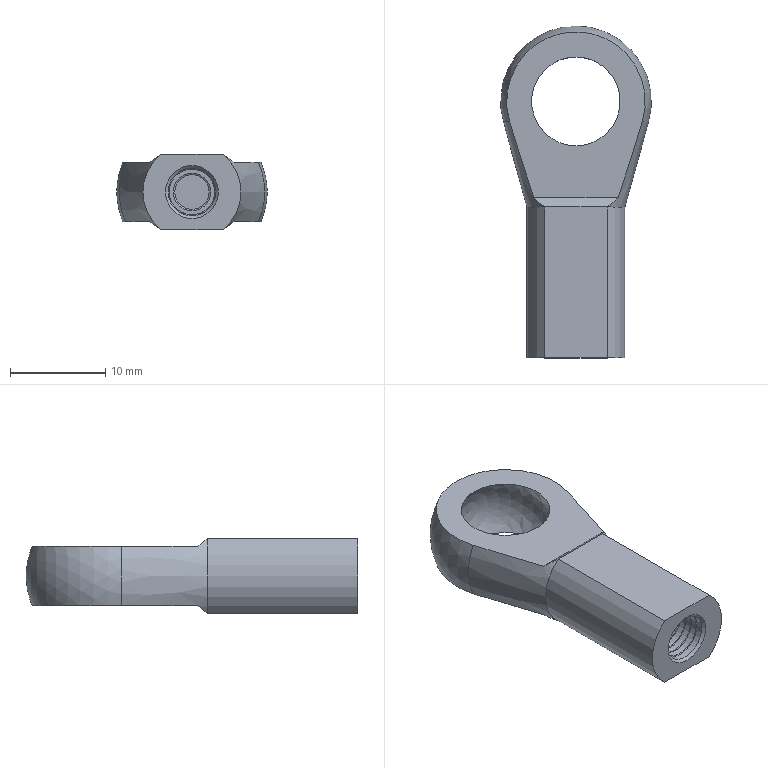Part | NX | features MG0312 tapped 1064K711(1064K711) 2 | 1 solid | 63 faces | box 15.875 x 34.925 x 7.925 mm | volume 1838 mm3 | cone 34 | cylinder 18 | plane 9 | sphere 2 | commonest cylinder face diameters 4.826 x15 10.312 x2 5 x1
STEP:
#1=CARTESIAN_POINT('',(6.982,12.167,-3.124));
#2=VERTEX_POINT('',#1);
#3=CARTESIAN_POINT('',(4.445,4.174,-3.124));
#4=VERTEX_POINT('',#3);
#5=CARTESIAN_POINT('',(6.982,12.167,-3.124));
#6=CARTESIAN_POINT('',(6.17,9.492,-3.124));
#7=CARTESIAN_POINT('',(5.342,6.821,-3.124));
#8=CARTESIAN_POINT('',(4.445,4.174,-3.124));
#9=B_SPLINE_CURVE_WITH_KNOTS('',3,(#5,#6,#7,#8),.UNSPECIFIED.,.F.,.F.,(4,4),(0.0111,0.01949),.UNSPECIFIED.);
#10=EDGE_CURVE('',#2,#4,#9,.T.);
#11=ORIENTED_EDGE('',*,*,#10,.F.);
#12=CARTESIAN_POINT('',(6.982,12.167,3.124));
#13=VERTEX_POINT('',#12);
#14=CARTESIAN_POINT('',(0.,12.167,0.));
#15=DIRECTION('',(0.,-1.,0.));
#16=DIRECTION('',(0.,0.,-1.));
#17=AXIS2_PLACEMENT_3D('',#14,#15,#16);
#18=CIRCLE('',#17,7.649);
#19=EDGE_CURVE('',#2,#13,#18,.T.);
#20=ORIENTED_EDGE('',*,*,#19,.T.);
#21=CARTESIAN_POINT('',(4.445,4.174,3.124));
#22=VERTEX_POINT('',#21);
#23=CARTESIAN_POINT('',(4.445,4.174,3.124));
#24=CARTESIAN_POINT('',(5.342,6.822,3.124));
#25=CARTESIAN_POINT('',(6.17,9.492,3.124));
#26=CARTESIAN_POINT('',(6.982,12.167,3.124));
#27=B_SPLINE_CURVE_WITH_KNOTS('',3,(#23,#24,#25,#26),.UNSPECIFIED.,.F.,.F.,(4,4),(0.03896,0.04741),.UNSPECIFIED.);
#28=EDGE_CURVE('',#22,#13,#27,.T.);
#29=ORIENTED_EDGE('',*,*,#28,.F.);
#30=CARTESIAN_POINT('',(3.299,3.175,3.962));
#31=VERTEX_POINT('',#30);
#32=CARTESIAN_POINT('',(0.,10.755,-2.398));
#33=DIRECTION('',(0.,0.6428,0.766));
#34=DIRECTION('',(0.,0.766,-0.6428));
#35=AXIS2_PLACEMENT_3D('',#32,#33,#34);
#36=ELLIPSE('',#35,11.291,6.85);
#37=EDGE_CURVE('',#22,#31,#36,.F.);
#38=ORIENTED_EDGE('',*,*,#37,.T.);
#39=CARTESIAN_POINT('',(3.299,3.175,-3.962));
#40=VERTEX_POINT('',#39);
#41=CARTESIAN_POINT('',(0.,3.175,0.));
#42=DIRECTION('',(0.,1.,0.));
#43=DIRECTION('',(0.,0.,1.));
#44=AXIS2_PLACEMENT_3D('',#41,#42,#43);
#45=CIRCLE('',#44,5.156);
#46=EDGE_CURVE('',#31,#40,#45,.T.);
#47=ORIENTED_EDGE('',*,*,#46,.T.);
#48=CARTESIAN_POINT('',(0.,10.755,2.398));
#49=DIRECTION('',(0.,0.6428,-0.766));
#50=DIRECTION('',(0.,0.766,0.6428));
#51=AXIS2_PLACEMENT_3D('',#48,#49,#50);
#52=ELLIPSE('',#51,11.291,6.85);
#53=EDGE_CURVE('',#40,#4,#52,.F.);
#54=ORIENTED_EDGE('',*,*,#53,.T.);
#55=EDGE_LOOP('',(#11,#20,#29,#38,#47,#54));
#56=FACE_BOUND('',#55,.T.);
#57=CARTESIAN_POINT('',(0.,3.175,0.));
#58=DIRECTION('',(0.,1.,0.));
#59=DIRECTION('',(0.,0.,1.));
#60=AXIS2_PLACEMENT_3D('',#57,#58,#59);
#61=CONICAL_SURFACE('',#60,5.156,0.2704);
#62=ADVANCED_FACE('',(#56),#61,.T.);
#63=CARTESIAN_POINT('',(-3.299,-12.7,-3.962));
#64=VERTEX_POINT('',#63);
#65=CARTESIAN_POINT('',(-3.299,3.175,-3.962));
#66=VERTEX_POINT('',#65);
#67=CARTESIAN_POINT('',(-3.299,22.225,-3.962));
#68=DIRECTION('',(0.,1.,0.));
#69=VECTOR('',#68,1000.);
#70=LINE('',#67,#69);
#71=EDGE_CURVE('',#64,#66,#70,.T.);
#72=ORIENTED_EDGE('',*,*,#71,.F.);
#73=CARTESIAN_POINT('',(-3.299,-12.7,3.962));
#74=VERTEX_POINT('',#73);
#75=CARTESIAN_POINT('',(0.,-12.7,0.));
#76=DIRECTION('',(0.,1.,0.));
#77=DIRECTION('',(0.,0.,1.));
#78=AXIS2_PLACEMENT_3D('',#75,#76,#77);
#79=CIRCLE('',#78,5.156);
#80=EDGE_CURVE('',#64,#74,#79,.T.);
#81=ORIENTED_EDGE('',*,*,#80,.T.);
#82=CARTESIAN_POINT('',(-3.299,3.175,3.962));
#83=VERTEX_POINT('',#82);
#84=CARTESIAN_POINT('',(-3.299,22.225,3.962));
#85=DIRECTION('',(0.,1.,0.));
#86=VECTOR('',#85,1000.);
#87=LINE('',#84,#86);
#88=EDGE_CURVE('',#83,#74,#87,.F.);
#89=ORIENTED_EDGE('',*,*,#88,.F.);
#90=CARTESIAN_POINT('',(0.,3.175,0.));
#91=DIRECTION('',(0.,1.,0.));
#92=DIRECTION('',(0.,0.,1.));
#93=AXIS2_PLACEMENT_3D('',#90,#91,#92);
#94=CIRCLE('',#93,5.156);
#95=EDGE_CURVE('',#66,#83,#94,.T.);
#96=ORIENTED_EDGE('',*,*,#95,.F.);
#97=EDGE_LOOP('',(#72,#81,#89,#96));
#98=FACE_BOUND('',#97,.T.);
#99=CARTESIAN_POINT('',(0.,22.225,0.));
#100=DIRECTION('',(0.,1.,0.));
#101=DIRECTION('',(0.,0.,1.));
#102=AXIS2_PLACEMENT_3D('',#99,#100,#101);
#103=CYLINDRICAL_SURFACE('',#102,5.156);
#104=ADVANCED_FACE('',(#98),#103,.T.);
#105=CARTESIAN_POINT('',(3.299,-12.7,-3.962));
#106=VERTEX_POINT('',#105);
#107=CARTESIAN_POINT('',(3.299,22.225,-3.962));
#108=DIRECTION('',(0.,1.,0.));
#109=VECTOR('',#108,1000.);
#110=LINE('',#107,#109);
#111=EDGE_CURVE('',#40,#106,#110,.F.);
#112=ORIENTED_EDGE('',*,*,#111,.F.);
#113=ORIENTED_EDGE('',*,*,#46,.F.);
#114=CARTESIAN_POINT('',(3.299,-12.7,3.962));
#115=VERTEX_POINT('',#114);
#116=CARTESIAN_POINT('',(3.299,22.225,3.962));
#117=DIRECTION('',(0.,1.,0.));
#118=VECTOR('',#117,1000.);
#119=LINE('',#116,#118);
#120=EDGE_CURVE('',#115,#31,#119,.T.);
#121=ORIENTED_EDGE('',*,*,#120,.F.);
#122=CARTESIAN_POINT('',(0.,-12.7,0.));
#123=DIRECTION('',(0.,1.,0.));
#124=DIRECTION('',(0.,0.,1.));
#125=AXIS2_PLACEMENT_3D('',#122,#123,#124);
#126=CIRCLE('',#125,5.156);
#127=EDGE_CURVE('',#115,#106,#126,.T.);
#128=ORIENTED_EDGE('',*,*,#127,.T.);
#129=EDGE_LOOP('',(#112,#113,#121,#128));
#130=FACE_BOUND('',#129,.T.);
#131=CARTESIAN_POINT('',(0.,22.225,0.));
#132=DIRECTION('',(0.,1.,0.));
#133=DIRECTION('',(0.,0.,1.));
#134=AXIS2_PLACEMENT_3D('',#131,#132,#133);
#135=CYLINDRICAL_SURFACE('',#134,5.156);
#136=ADVANCED_FACE('',(#130),#135,.T.);
#137=CARTESIAN_POINT('',(2.788,-12.7,0.));
#138=VERTEX_POINT('',#137);
#139=CARTESIAN_POINT('',(0.,-12.7,0.));
#140=DIRECTION('',(0.,-1.,0.));
#141=DIRECTION('',(1.,0.,0.));
#142=AXIS2_PLACEMENT_3D('',#139,#140,#141);
#143=CIRCLE('',#142,2.788);
#144=EDGE_CURVE('',#138,#138,#143,.T.);
#145=ORIENTED_EDGE('',*,*,#144,.F.);
#146=EDGE_LOOP('',(#145));
#147=FACE_BOUND('',#146,.T.);
#148=CARTESIAN_POINT('',(5.156,-12.7,-3.962));
#149=DIRECTION('',(-1.,0.,0.));
#150=VECTOR('',#149,1000.);
#151=LINE('',#148,#150);
#152=EDGE_CURVE('',#106,#64,#151,.T.);
#153=ORIENTED_EDGE('',*,*,#152,.F.);
#154=ORIENTED_EDGE('',*,*,#127,.F.);
#155=CARTESIAN_POINT('',(5.156,-12.7,3.962));
#156=DIRECTION('',(1.,0.,0.));
#157=VECTOR('',#156,1000.);
#158=LINE('',#155,#157);
#159=EDGE_CURVE('',#74,#115,#158,.T.);
#160=ORIENTED_EDGE('',*,*,#159,.F.);
#161=ORIENTED_EDGE('',*,*,#80,.F.);
#162=EDGE_LOOP('',(#153,#154,#160,#161));
#163=FACE_BOUND('',#162,.T.);
#164=CARTESIAN_POINT('',(5.156,-12.7,0.));
#165=DIRECTION('',(0.,1.,0.));
#166=DIRECTION('',(0.,0.,1.));
#167=AXIS2_PLACEMENT_3D('',#164,#165,#166);
#168=PLANE('',#167);
#169=ADVANCED_FACE('',(#147,#163),#168,.F.);
#170=ORIENTED_EDGE('',*,*,#120,.T.);
#171=CARTESIAN_POINT('',(-3.962,3.175,3.962));
#172=DIRECTION('',(-1.,0.,0.));
#173=VECTOR('',#172,1000.);
#174=LINE('',#171,#173);
#175=EDGE_CURVE('',#31,#83,#174,.T.);
#176=ORIENTED_EDGE('',*,*,#175,.T.);
#177=ORIENTED_EDGE('',*,*,#88,.T.);
#178=ORIENTED_EDGE('',*,*,#159,.T.);
#179=EDGE_LOOP('',(#170,#176,#177,#178));
#180=FACE_BOUND('',#179,.T.);
#181=CARTESIAN_POINT('',(-3.962,3.175,3.962));
#182=DIRECTION('',(0.,0.,1.));
#183=DIRECTION('',(1.,0.,0.));
#184=AXIS2_PLACEMENT_3D('',#181,#182,#183);
#185=PLANE('',#184);
#186=ADVANCED_FACE('',(#180),#185,.T.);
#187=ORIENTED_EDGE('',*,*,#71,.T.);
#188=CARTESIAN_POINT('',(-3.962,3.175,-3.962));
#189=DIRECTION('',(1.,0.,0.));
#190=VECTOR('',#189,1000.);
#191=LINE('',#188,#190);
#192=EDGE_CURVE('',#66,#40,#191,.T.);
#193=ORIENTED_EDGE('',*,*,#192,.T.);
#194=ORIENTED_EDGE('',*,*,#111,.T.);
#195=ORIENTED_EDGE('',*,*,#152,.T.);
#196=EDGE_LOOP('',(#187,#193,#194,#195));
#197=FACE_BOUND('',#196,.T.);
#198=CARTESIAN_POINT('',(-3.962,3.175,-3.962));
#199=DIRECTION('',(0.,0.,-1.));
#200=DIRECTION('',(-1.,0.,0.));
#201=AXIS2_PLACEMENT_3D('',#198,#199,#200);
#202=PLANE('',#201);
#203=ADVANCED_FACE('',(#197),#202,.T.);
#204=CARTESIAN_POINT('',(2.5,-12.412,0.));
#205=VERTEX_POINT('',#204);
#206=CARTESIAN_POINT('',(0.,-12.412,0.));
#207=DIRECTION('',(0.,-1.,0.));
#208=DIRECTION('',(1.,0.,0.));
#209=AXIS2_PLACEMENT_3D('',#206,#207,#208);
#210=CIRCLE('',#209,2.5);
#211=EDGE_CURVE('',#205,#205,#210,.F.);
#212=ORIENTED_EDGE('',*,*,#211,.T.);
#213=EDGE_LOOP('',(#212));
#214=FACE_BOUND('',#213,.T.);
#215=ORIENTED_EDGE('',*,*,#144,.T.);
#216=EDGE_LOOP('',(#215));
#217=FACE_BOUND('',#216,.T.);
#218=CARTESIAN_POINT('',(0.,-12.7,0.));
#219=DIRECTION('',(0.,-1.,0.));
#220=DIRECTION('',(1.,0.,0.));
#221=AXIS2_PLACEMENT_3D('',#218,#219,#220);
#222=CONICAL_SURFACE('',#221,2.788,0.7854);
#223=ADVANCED_FACE('',(#214,#217),#222,.F.);
#224=CARTESIAN_POINT('',(-4.445,4.174,-3.124));
#225=VERTEX_POINT('',#224);
#226=CARTESIAN_POINT('',(-6.982,12.167,-3.124));
#227=VERTEX_POINT('',#226);
#228=CARTESIAN_POINT('',(-4.445,4.174,-3.124));
#229=CARTESIAN_POINT('',(-5.342,6.822,-3.124));
#230=CARTESIAN_POINT('',(-6.17,9.492,-3.124));
#231=CARTESIAN_POINT('',(-6.982,12.167,-3.124));
#232=B_SPLINE_CURVE_WITH_KNOTS('',3,(#228,#229,#230,#231),.UNSPECIFIED.,.F.,.F.,(4,4),(0.03896,0.04741),.UNSPECIFIED.);
#233=EDGE_CURVE('',#225,#227,#232,.T.);
#234=ORIENTED_EDGE('',*,*,#233,.F.);
#235=CARTESIAN_POINT('',(0.,10.755,2.398));
#236=DIRECTION('',(0.,0.6428,-0.766));
#237=DIRECTION('',(0.,0.766,0.6428));
#238=AXIS2_PLACEMENT_3D('',#235,#236,#237);
#239=ELLIPSE('',#238,11.291,6.85);
#240=EDGE_CURVE('',#225,#66,#239,.F.);
#241=ORIENTED_EDGE('',*,*,#240,.T.);
#242=ORIENTED_EDGE('',*,*,#95,.T.);
#243=CARTESIAN_POINT('',(-4.445,4.174,3.124));
#244=VERTEX_POINT('',#243);
#245=CARTESIAN_POINT('',(0.,10.755,-2.398));
#246=DIRECTION('',(0.,0.6428,0.766));
#247=DIRECTION('',(0.,0.766,-0.6428));
#248=AXIS2_PLACEMENT_3D('',#245,#246,#247);
#249=ELLIPSE('',#248,11.291,6.85);
#250=EDGE_CURVE('',#83,#244,#249,.F.);
#251=ORIENTED_EDGE('',*,*,#250,.T.);
#252=CARTESIAN_POINT('',(-6.982,12.167,3.124));
#253=VERTEX_POINT('',#252);
#254=CARTESIAN_POINT('',(-6.982,12.167,3.124));
#255=CARTESIAN_POINT('',(-6.17,9.492,3.124));
#256=CARTESIAN_POINT('',(-5.342,6.821,3.124));
#257=CARTESIAN_POINT('',(-4.445,4.174,3.124));
#258=B_SPLINE_CURVE_WITH_KNOTS('',3,(#254,#255,#256,#257),.UNSPECIFIED.,.F.,.F.,(4,4),(0.0111,0.01949),.UNSPECIFIED.);
#259=EDGE_CURVE('',#253,#244,#258,.T.);
#260=ORIENTED_EDGE('',*,*,#259,.F.);
#261=CARTESIAN_POINT('',(0.,12.167,0.));
#262=DIRECTION('',(0.,-1.,0.));
#263=DIRECTION('',(0.,0.,-1.));
#264=AXIS2_PLACEMENT_3D('',#261,#262,#263);
#265=CIRCLE('',#264,7.649);
#266=EDGE_CURVE('',#253,#227,#265,.T.);
#267=ORIENTED_EDGE('',*,*,#266,.T.);
#268=EDGE_LOOP('',(#234,#241,#242,#251,#260,#267));
#269=FACE_BOUND('',#268,.T.);
#270=CARTESIAN_POINT('',(0.,3.175,0.));
#271=DIRECTION('',(0.,1.,0.));
#272=DIRECTION('',(0.,0.,1.));
#273=AXIS2_PLACEMENT_3D('',#270,#271,#272);
#274=CONICAL_SURFACE('',#273,5.156,0.2704);
#275=ADVANCED_FACE('',(#269),#274,.T.);
#276=CARTESIAN_POINT('',(0.,14.287,-3.124));
#277=DIRECTION('',(0.,0.,1.));
#278=DIRECTION('',(0.,-1.,0.));
#279=AXIS2_PLACEMENT_3D('',#276,#277,#278);
#280=CIRCLE('',#279,7.297);
#281=EDGE_CURVE('',#227,#2,#280,.F.);
#282=ORIENTED_EDGE('',*,*,#281,.F.);
#283=ORIENTED_EDGE('',*,*,#266,.F.);
#284=CARTESIAN_POINT('',(0.,14.287,3.124));
#285=DIRECTION('',(0.,0.,-1.));
#286=DIRECTION('',(0.,1.,0.));
#287=AXIS2_PLACEMENT_3D('',#284,#285,#286);
#288=CIRCLE('',#287,7.297);
#289=EDGE_CURVE('',#13,#253,#288,.F.);
#290=ORIENTED_EDGE('',*,*,#289,.F.);
#291=ORIENTED_EDGE('',*,*,#19,.F.);
#292=EDGE_LOOP('',(#282,#283,#290,#291));
#293=FACE_BOUND('',#292,.T.);
#294=CARTESIAN_POINT('',(0.,14.287,0.));
#295=DIRECTION('',(0.,-1.,0.));
#296=DIRECTION('',(1.,0.,0.));
#297=AXIS2_PLACEMENT_3D('',#294,#295,#296);
#298=SPHERICAL_SURFACE('',#297,7.938);
#299=ADVANCED_FACE('',(#293),#298,.T.);
#300=CARTESIAN_POINT('',(0.,18.957,3.124));
#301=VERTEX_POINT('',#300);
#302=CARTESIAN_POINT('',(0.,14.287,3.124));
#303=DIRECTION('',(0.,0.,-1.));
#304=DIRECTION('',(0.,1.,0.));
#305=AXIS2_PLACEMENT_3D('',#302,#303,#304);
#306=CIRCLE('',#305,4.669);
#307=EDGE_CURVE('',#301,#301,#306,.F.);
#308=ORIENTED_EDGE('',*,*,#307,.F.);
#309=EDGE_LOOP('',(#308));
#310=FACE_BOUND('',#309,.T.);
#311=ORIENTED_EDGE('',*,*,#259,.T.);
#312=CARTESIAN_POINT('',(4.102,4.174,3.124));
#313=DIRECTION('',(1.,0.,0.));
#314=VECTOR('',#313,1000.);
#315=LINE('',#312,#314);
#316=EDGE_CURVE('',#244,#22,#315,.T.);
#317=ORIENTED_EDGE('',*,*,#316,.T.);
#318=ORIENTED_EDGE('',*,*,#28,.T.);
#319=ORIENTED_EDGE('',*,*,#289,.T.);
#320=EDGE_LOOP('',(#311,#317,#318,#319));
#321=FACE_BOUND('',#320,.T.);
#322=CARTESIAN_POINT('',(-7.938,22.225,3.124));
#323=DIRECTION('',(0.,0.,-1.));
#324=DIRECTION('',(0.,1.,0.));
#325=AXIS2_PLACEMENT_3D('',#322,#323,#324);
#326=PLANE('',#325);
#327=ADVANCED_FACE('',(#310,#321),#326,.F.);
#328=CARTESIAN_POINT('',(0.,9.618,-3.124));
#329=VERTEX_POINT('',#328);
#330=CARTESIAN_POINT('',(0.,14.287,-3.124));
#331=DIRECTION('',(0.,0.,1.));
#332=DIRECTION('',(0.,-1.,0.));
#333=AXIS2_PLACEMENT_3D('',#330,#331,#332);
#334=CIRCLE('',#333,4.669);
#335=EDGE_CURVE('',#329,#329,#334,.F.);
#336=ORIENTED_EDGE('',*,*,#335,.F.);
#337=EDGE_LOOP('',(#336));
#338=FACE_BOUND('',#337,.T.);
#339=ORIENTED_EDGE('',*,*,#10,.T.);
#340=CARTESIAN_POINT('',(-4.102,4.174,-3.124));
#341=DIRECTION('',(-1.,0.,0.));
#342=VECTOR('',#341,1000.);
#343=LINE('',#340,#342);
#344=EDGE_CURVE('',#4,#225,#343,.T.);
#345=ORIENTED_EDGE('',*,*,#344,.T.);
#346=ORIENTED_EDGE('',*,*,#233,.T.);
#347=ORIENTED_EDGE('',*,*,#281,.T.);
#348=EDGE_LOOP('',(#339,#345,#346,#347));
#349=FACE_BOUND('',#348,.T.);
#350=CARTESIAN_POINT('',(-7.938,22.225,-3.124));
#351=DIRECTION('',(0.,0.,1.));
#352=DIRECTION('',(0.,-1.,0.));
#353=AXIS2_PLACEMENT_3D('',#350,#351,#352);
#354=PLANE('',#353);
#355=ADVANCED_FACE('',(#338,#349),#354,.F.);
#356=ORIENTED_EDGE('',*,*,#240,.F.);
#357=ORIENTED_EDGE('',*,*,#344,.F.);
#358=ORIENTED_EDGE('',*,*,#53,.F.);
#359=ORIENTED_EDGE('',*,*,#192,.F.);
#360=EDGE_LOOP('',(#356,#357,#358,#359));
#361=FACE_BOUND('',#360,.T.);
#362=CARTESIAN_POINT('',(-7.938,3.175,-3.962));
#363=DIRECTION('',(0.,0.6428,-0.766));
#364=DIRECTION('',(0.,0.766,0.6428));
#365=AXIS2_PLACEMENT_3D('',#362,#363,#364);
#366=PLANE('',#365);
#367=ADVANCED_FACE('',(#361),#366,.T.);
#368=ORIENTED_EDGE('',*,*,#250,.F.);
#369=ORIENTED_EDGE('',*,*,#175,.F.);
#370=ORIENTED_EDGE('',*,*,#37,.F.);
#371=ORIENTED_EDGE('',*,*,#316,.F.);
#372=EDGE_LOOP('',(#368,#369,#370,#371));
#373=FACE_BOUND('',#372,.T.);
#374=CARTESIAN_POINT('',(-7.938,4.174,3.124));
#375=DIRECTION('',(0.,0.6428,0.766));
#376=DIRECTION('',(0.,-0.766,0.6428));
#377=AXIS2_PLACEMENT_3D('',#374,#375,#376);
#378=PLANE('',#377);
#379=ADVANCED_FACE('',(#373),#378,.T.);
#380=ORIENTED_EDGE('',*,*,#335,.T.);
#381=EDGE_LOOP('',(#380));
#382=FACE_BOUND('',#381,.T.);
#383=ORIENTED_EDGE('',*,*,#307,.T.);
#384=EDGE_LOOP('',(#383));
#385=FACE_BOUND('',#384,.T.);
#386=CARTESIAN_POINT('',(0.,14.287,0.));
#387=DIRECTION('',(0.,1.,0.));
#388=DIRECTION('',(1.,0.,0.));
#389=AXIS2_PLACEMENT_3D('',#386,#387,#388);
#390=SPHERICAL_SURFACE('',#389,5.618);
#391=ADVANCED_FACE('',(#382,#385),#390,.F.);
#392=CARTESIAN_POINT('',(2.5,-11.7,0.));
#393=VERTEX_POINT('',#392);
#394=CARTESIAN_POINT('',(0.,-11.7,0.));
#395=DIRECTION('',(0.,-1.,0.));
#396=DIRECTION('',(1.,0.,0.));
#397=AXIS2_PLACEMENT_3D('',#394,#395,#396);
#398=CIRCLE('',#397,2.5);
#399=EDGE_CURVE('',#393,#393,#398,.T.);
#400=ORIENTED_EDGE('',*,*,#399,.F.);
#401=EDGE_LOOP('',(#400));
#402=FACE_BOUND('',#401,.T.);
#403=ORIENTED_EDGE('',*,*,#211,.F.);
#404=EDGE_LOOP('',(#403));
#405=FACE_BOUND('',#404,.T.);
#406=CARTESIAN_POINT('',(0.,-12.7,0.));
#407=DIRECTION('',(0.,-1.,0.));
#408=DIRECTION('',(1.,0.,0.));
#409=AXIS2_PLACEMENT_3D('',#406,#407,#408);
#410=CYLINDRICAL_SURFACE('',#409,2.5);
#411=ADVANCED_FACE('',(#402,#405),#410,.F.);
#412=ORIENTED_EDGE('',*,*,#399,.T.);
#413=EDGE_LOOP('',(#412));
#414=FACE_BOUND('',#413,.T.);
#415=CARTESIAN_POINT('',(2.413,-11.65,0.));
#416=VERTEX_POINT('',#415);
#417=CARTESIAN_POINT('',(0.,-11.65,0.));
#418=DIRECTION('',(0.,-1.,0.));
#419=DIRECTION('',(1.,0.,0.));
#420=AXIS2_PLACEMENT_3D('',#417,#418,#419);
#421=CIRCLE('',#420,2.413);
#422=EDGE_CURVE('',#416,#416,#421,.T.);
#423=ORIENTED_EDGE('',*,*,#422,.F.);
#424=EDGE_LOOP('',(#423));
#425=FACE_BOUND('',#424,.T.);
#426=CARTESIAN_POINT('',(0.,-11.7,0.));
#427=DIRECTION('',(0.,-1.,0.));
#428=DIRECTION('',(1.,0.,0.));
#429=AXIS2_PLACEMENT_3D('',#426,#427,#428);
#430=CONICAL_SURFACE('',#429,2.5,1.047);
#431=ADVANCED_FACE('',(#414,#425),#430,.F.);
#432=ORIENTED_EDGE('',*,*,#422,.T.);
#433=EDGE_LOOP('',(#432));
#434=FACE_BOUND('',#433,.T.);
#435=CARTESIAN_POINT('',(-2.413,-10.95,0.));
#436=VERTEX_POINT('',#435);
#437=CARTESIAN_POINT('',(0.,-10.95,0.));
#438=DIRECTION('',(0.,1.,0.));
#439=DIRECTION('',(-1.,0.,0.));
#440=AXIS2_PLACEMENT_3D('',#437,#438,#439);
#441=CIRCLE('',#440,2.413);
#442=EDGE_CURVE('',#436,#436,#441,.T.);
#443=ORIENTED_EDGE('',*,*,#442,.T.);
#444=EDGE_LOOP('',(#443));
#445=FACE_BOUND('',#444,.T.);
#446=CARTESIAN_POINT('',(0.,0.,0.));
#447=DIRECTION('',(0.,-1.,0.));
#448=DIRECTION('',(0.,0.,-1.));
#449=AXIS2_PLACEMENT_3D('',#446,#447,#448);
#450=CYLINDRICAL_SURFACE('',#449,2.413);
#451=ADVANCED_FACE('',(#434,#445),#450,.F.);
#452=CARTESIAN_POINT('',(2.5,-10.9,0.));
#453=VERTEX_POINT('',#452);
#454=CARTESIAN_POINT('',(0.,-10.9,0.));
#455=DIRECTION('',(0.,-1.,0.));
#456=DIRECTION('',(1.,0.,0.));
#457=AXIS2_PLACEMENT_3D('',#454,#455,#456);
#458=CIRCLE('',#457,2.5);
#459=EDGE_CURVE('',#453,#453,#458,.T.);
#460=ORIENTED_EDGE('',*,*,#459,.T.);
#461=EDGE_LOOP('',(#460));
#462=FACE_BOUND('',#461,.T.);
#463=CARTESIAN_POINT('',(2.413,-10.85,0.));
#464=VERTEX_POINT('',#463);
#465=CARTESIAN_POINT('',(0.,-10.85,0.));
#466=DIRECTION('',(0.,-1.,0.));
#467=DIRECTION('',(1.,0.,0.));
#468=AXIS2_PLACEMENT_3D('',#465,#466,#467);
#469=CIRCLE('',#468,2.413);
#470=EDGE_CURVE('',#464,#464,#469,.T.);
#471=ORIENTED_EDGE('',*,*,#470,.F.);
#472=EDGE_LOOP('',(#471));
#473=FACE_BOUND('',#472,.T.);
#474=CARTESIAN_POINT('',(0.,-10.9,0.));
#475=DIRECTION('',(0.,-1.,0.));
#476=DIRECTION('',(1.,0.,0.));
#477=AXIS2_PLACEMENT_3D('',#474,#475,#476);
#478=CONICAL_SURFACE('',#477,2.5,1.047);
#479=ADVANCED_FACE('',(#462,#473),#478,.F.);
#480=ORIENTED_EDGE('',*,*,#459,.F.);
#481=EDGE_LOOP('',(#480));
#482=FACE_BOUND('',#481,.T.);
#483=ORIENTED_EDGE('',*,*,#442,.F.);
#484=EDGE_LOOP('',(#483));
#485=FACE_BOUND('',#484,.T.);
#486=CARTESIAN_POINT('',(0.,-11.3,0.));
#487=DIRECTION('',(0.,1.,0.));
#488=DIRECTION('',(-1.,0.,0.));
#489=AXIS2_PLACEMENT_3D('',#486,#487,#488);
#490=CONICAL_SURFACE('',#489,1.807,1.047);
#491=ADVANCED_FACE('',(#482,#485),#490,.F.);
#492=ORIENTED_EDGE('',*,*,#470,.T.);
#493=EDGE_LOOP('',(#492));
#494=FACE_BOUND('',#493,.T.);
#495=CARTESIAN_POINT('',(-2.413,-10.15,0.));
#496=VERTEX_POINT('',#495);
#497=CARTESIAN_POINT('',(0.,-10.15,0.));
#498=DIRECTION('',(0.,1.,0.));
#499=DIRECTION('',(-1.,0.,0.));
#500=AXIS2_PLACEMENT_3D('',#497,#498,#499);
#501=CIRCLE('',#500,2.413);
#502=EDGE_CURVE('',#496,#496,#501,.T.);
#503=ORIENTED_EDGE('',*,*,#502,.T.);
#504=EDGE_LOOP('',(#503));
#505=FACE_BOUND('',#504,.T.);
#506=CARTESIAN_POINT('',(0.,0.,0.));
#507=DIRECTION('',(0.,-1.,0.));
#508=DIRECTION('',(0.,0.,-1.));
#509=AXIS2_PLACEMENT_3D('',#506,#507,#508);
#510=CYLINDRICAL_SURFACE('',#509,2.413);
#511=ADVANCED_FACE('',(#494,#505),#510,.F.);
#512=CARTESIAN_POINT('',(2.5,-10.1,0.));
#513=VERTEX_POINT('',#512);
#514=CARTESIAN_POINT('',(0.,-10.1,0.));
#515=DIRECTION('',(0.,-1.,0.));
#516=DIRECTION('',(1.,0.,0.));
#517=AXIS2_PLACEMENT_3D('',#514,#515,#516);
#518=CIRCLE('',#517,2.5);
#519=EDGE_CURVE('',#513,#513,#518,.T.);
#520=ORIENTED_EDGE('',*,*,#519,.T.);
#521=EDGE_LOOP('',(#520));
#522=FACE_BOUND('',#521,.T.);
#523=CARTESIAN_POINT('',(2.413,-10.05,0.));
#524=VERTEX_POINT('',#523);
#525=CARTESIAN_POINT('',(0.,-10.05,0.));
#526=DIRECTION('',(0.,-1.,0.));
#527=DIRECTION('',(1.,0.,0.));
#528=AXIS2_PLACEMENT_3D('',#525,#526,#527);
#529=CIRCLE('',#528,2.413);
#530=EDGE_CURVE('',#524,#524,#529,.T.);
#531=ORIENTED_EDGE('',*,*,#530,.F.);
#532=EDGE_LOOP('',(#531));
#533=FACE_BOUND('',#532,.T.);
#534=CARTESIAN_POINT('',(0.,-10.1,0.));
#535=DIRECTION('',(0.,-1.,0.));
#536=DIRECTION('',(1.,0.,0.));
#537=AXIS2_PLACEMENT_3D('',#534,#535,#536);
#538=CONICAL_SURFACE('',#537,2.5,1.047);
#539=ADVANCED_FACE('',(#522,#533),#538,.F.);
#540=ORIENTED_EDGE('',*,*,#519,.F.);
#541=EDGE_LOOP('',(#540));
#542=FACE_BOUND('',#541,.T.);
#543=ORIENTED_EDGE('',*,*,#502,.F.);
#544=EDGE_LOOP('',(#543));
#545=FACE_BOUND('',#544,.T.);
#546=CARTESIAN_POINT('',(0.,-10.5,0.));
#547=DIRECTION('',(0.,1.,0.));
#548=DIRECTION('',(-1.,0.,0.));
#549=AXIS2_PLACEMENT_3D('',#546,#547,#548);
#550=CONICAL_SURFACE('',#549,1.807,1.047);
#551=ADVANCED_FACE('',(#542,#545),#550,.F.);
#552=ORIENTED_EDGE('',*,*,#530,.T.);
#553=EDGE_LOOP('',(#552));
#554=FACE_BOUND('',#553,.T.);
#555=CARTESIAN_POINT('',(-2.413,-9.35,0.));
#556=VERTEX_POINT('',#555);
#557=CARTESIAN_POINT('',(0.,-9.35,0.));
#558=DIRECTION('',(0.,1.,0.));
#559=DIRECTION('',(-1.,0.,0.));
#560=AXIS2_PLACEMENT_3D('',#557,#558,#559);
#561=CIRCLE('',#560,2.413);
#562=EDGE_CURVE('',#556,#556,#561,.T.);
#563=ORIENTED_EDGE('',*,*,#562,.T.);
#564=EDGE_LOOP('',(#563));
#565=FACE_BOUND('',#564,.T.);
#566=CARTESIAN_POINT('',(0.,0.,0.));
#567=DIRECTION('',(0.,-1.,0.));
#568=DIRECTION('',(0.,0.,-1.));
#569=AXIS2_PLACEMENT_3D('',#566,#567,#568);
#570=CYLINDRICAL_SURFACE('',#569,2.413);
#571=ADVANCED_FACE('',(#554,#565),#570,.F.);
#572=CARTESIAN_POINT('',(2.5,-9.3,0.));
#573=VERTEX_POINT('',#572);
#574=CARTESIAN_POINT('',(0.,-9.3,0.));
#575=DIRECTION('',(0.,-1.,0.));
#576=DIRECTION('',(1.,0.,0.));
#577=AXIS2_PLACEMENT_3D('',#574,#575,#576);
#578=CIRCLE('',#577,2.5);
#579=EDGE_CURVE('',#573,#573,#578,.T.);
#580=ORIENTED_EDGE('',*,*,#579,.T.);
#581=EDGE_LOOP('',(#580));
#582=FACE_BOUND('',#581,.T.);
#583=CARTESIAN_POINT('',(2.413,-9.25,0.));
#584=VERTEX_POINT('',#583);
#585=CARTESIAN_POINT('',(0.,-9.25,0.));
#586=DIRECTION('',(0.,-1.,0.));
#587=DIRECTION('',(1.,0.,0.));
#588=AXIS2_PLACEMENT_3D('',#585,#586,#587);
#589=CIRCLE('',#588,2.413);
#590=EDGE_CURVE('',#584,#584,#589,.T.);
#591=ORIENTED_EDGE('',*,*,#590,.F.);
#592=EDGE_LOOP('',(#591));
#593=FACE_BOUND('',#592,.T.);
#594=CARTESIAN_POINT('',(0.,-9.3,0.));
#595=DIRECTION('',(0.,-1.,0.));
#596=DIRECTION('',(1.,0.,0.));
#597=AXIS2_PLACEMENT_3D('',#594,#595,#596);
#598=CONICAL_SURFACE('',#597,2.5,1.047);
#599=ADVANCED_FACE('',(#582,#593),#598,.F.);
#600=ORIENTED_EDGE('',*,*,#579,.F.);
#601=EDGE_LOOP('',(#600));
#602=FACE_BOUND('',#601,.T.);
#603=ORIENTED_EDGE('',*,*,#562,.F.);
#604=EDGE_LOOP('',(#603));
#605=FACE_BOUND('',#604,.T.);
#606=CARTESIAN_POINT('',(0.,-9.7,0.));
#607=DIRECTION('',(0.,1.,0.));
#608=DIRECTION('',(-1.,0.,0.));
#609=AXIS2_PLACEMENT_3D('',#606,#607,#608);
#610=CONICAL_SURFACE('',#609,1.807,1.047);
#611=ADVANCED_FACE('',(#602,#605),#610,.F.);
#612=ORIENTED_EDGE('',*,*,#590,.T.);
#613=EDGE_LOOP('',(#612));
#614=FACE_BOUND('',#613,.T.);
#615=CARTESIAN_POINT('',(-2.413,-8.55,0.));
#616=VERTEX_POINT('',#615);
#617=CARTESIAN_POINT('',(0.,-8.55,0.));
#618=DIRECTION('',(0.,1.,0.));
#619=DIRECTION('',(-1.,0.,0.));
#620=AXIS2_PLACEMENT_3D('',#617,#618,#619);
#621=CIRCLE('',#620,2.413);
#622=EDGE_CURVE('',#616,#616,#621,.T.);
#623=ORIENTED_EDGE('',*,*,#622,.T.);
#624=EDGE_LOOP('',(#623));
#625=FACE_BOUND('',#624,.T.);
#626=CARTESIAN_POINT('',(0.,0.,0.));
#627=DIRECTION('',(0.,-1.,0.));
#628=DIRECTION('',(0.,0.,-1.));
#629=AXIS2_PLACEMENT_3D('',#626,#627,#628);
#630=CYLINDRICAL_SURFACE('',#629,2.413);
#631=ADVANCED_FACE('',(#614,#625),#630,.F.);
#632=CARTESIAN_POINT('',(2.5,-8.5,0.));
#633=VERTEX_POINT('',#632);
#634=CARTESIAN_POINT('',(0.,-8.5,0.));
#635=DIRECTION('',(0.,-1.,0.));
#636=DIRECTION('',(1.,0.,0.));
#637=AXIS2_PLACEMENT_3D('',#634,#635,#636);
#638=CIRCLE('',#637,2.5);
#639=EDGE_CURVE('',#633,#633,#638,.T.);
#640=ORIENTED_EDGE('',*,*,#639,.T.);
#641=EDGE_LOOP('',(#640));
#642=FACE_BOUND('',#641,.T.);
#643=CARTESIAN_POINT('',(2.413,-8.45,0.));
#644=VERTEX_POINT('',#643);
#645=CARTESIAN_POINT('',(0.,-8.45,0.));
#646=DIRECTION('',(0.,-1.,0.));
#647=DIRECTION('',(1.,0.,0.));
#648=AXIS2_PLACEMENT_3D('',#645,#646,#647);
#649=CIRCLE('',#648,2.413);
#650=EDGE_CURVE('',#644,#644,#649,.T.);
#651=ORIENTED_EDGE('',*,*,#650,.F.);
#652=EDGE_LOOP('',(#651));
#653=FACE_BOUND('',#652,.T.);
#654=CARTESIAN_POINT('',(0.,-8.5,0.));
#655=DIRECTION('',(0.,-1.,0.));
#656=DIRECTION('',(1.,0.,0.));
#657=AXIS2_PLACEMENT_3D('',#654,#655,#656);
#658=CONICAL_SURFACE('',#657,2.5,1.047);
#659=ADVANCED_FACE('',(#642,#653),#658,.F.);
#660=ORIENTED_EDGE('',*,*,#639,.F.);
#661=EDGE_LOOP('',(#660));
#662=FACE_BOUND('',#661,.T.);
#663=ORIENTED_EDGE('',*,*,#622,.F.);
#664=EDGE_LOOP('',(#663));
#665=FACE_BOUND('',#664,.T.);
#666=CARTESIAN_POINT('',(0.,-8.9,0.));
#667=DIRECTION('',(0.,1.,0.));
#668=DIRECTION('',(-1.,0.,0.));
#669=AXIS2_PLACEMENT_3D('',#666,#667,#668);
#670=CONICAL_SURFACE('',#669,1.807,1.047);
#671=ADVANCED_FACE('',(#662,#665),#670,.F.);
#672=ORIENTED_EDGE('',*,*,#650,.T.);
#673=EDGE_LOOP('',(#672));
#674=FACE_BOUND('',#673,.T.);
#675=CARTESIAN_POINT('',(-2.413,-7.75,0.));
#676=VERTEX_POINT('',#675);
#677=CARTESIAN_POINT('',(0.,-7.75,0.));
#678=DIRECTION('',(0.,1.,0.));
#679=DIRECTION('',(-1.,0.,0.));
#680=AXIS2_PLACEMENT_3D('',#677,#678,#679);
#681=CIRCLE('',#680,2.413);
#682=EDGE_CURVE('',#676,#676,#681,.T.);
#683=ORIENTED_EDGE('',*,*,#682,.T.);
#684=EDGE_LOOP('',(#683));
#685=FACE_BOUND('',#684,.T.);
#686=CARTESIAN_POINT('',(0.,0.,0.));
#687=DIRECTION('',(0.,-1.,0.));
#688=DIRECTION('',(0.,0.,-1.));
#689=AXIS2_PLACEMENT_3D('',#686,#687,#688);
#690=CYLINDRICAL_SURFACE('',#689,2.413);
#691=ADVANCED_FACE('',(#674,#685),#690,.F.);
#692=CARTESIAN_POINT('',(2.5,-7.7,0.));
#693=VERTEX_POINT('',#692);
#694=CARTESIAN_POINT('',(0.,-7.7,0.));
#695=DIRECTION('',(0.,-1.,0.));
#696=DIRECTION('',(1.,0.,0.));
#697=AXIS2_PLACEMENT_3D('',#694,#695,#696);
#698=CIRCLE('',#697,2.5);
#699=EDGE_CURVE('',#693,#693,#698,.T.);
#700=ORIENTED_EDGE('',*,*,#699,.T.);
#701=EDGE_LOOP('',(#700));
#702=FACE_BOUND('',#701,.T.);
#703=CARTESIAN_POINT('',(2.413,-7.65,0.));
#704=VERTEX_POINT('',#703);
#705=CARTESIAN_POINT('',(0.,-7.65,0.));
#706=DIRECTION('',(0.,-1.,0.));
#707=DIRECTION('',(1.,0.,0.));
#708=AXIS2_PLACEMENT_3D('',#705,#706,#707);
#709=CIRCLE('',#708,2.413);
#710=EDGE_CURVE('',#704,#704,#709,.T.);
#711=ORIENTED_EDGE('',*,*,#710,.F.);
#712=EDGE_LOOP('',(#711));
#713=FACE_BOUND('',#712,.T.);
#714=CARTESIAN_POINT('',(0.,-7.7,0.));
#715=DIRECTION('',(0.,-1.,0.));
#716=DIRECTION('',(1.,0.,0.));
#717=AXIS2_PLACEMENT_3D('',#714,#715,#716);
#718=CONICAL_SURFACE('',#717,2.5,1.047);
#719=ADVANCED_FACE('',(#702,#713),#718,.F.);
#720=ORIENTED_EDGE('',*,*,#699,.F.);
#721=EDGE_LOOP('',(#720));
#722=FACE_BOUND('',#721,.T.);
#723=ORIENTED_EDGE('',*,*,#682,.F.);
#724=EDGE_LOOP('',(#723));
#725=FACE_BOUND('',#724,.T.);
#726=CARTESIAN_POINT('',(0.,-8.1,0.));
#727=DIRECTION('',(0.,1.,0.));
#728=DIRECTION('',(-1.,0.,0.));
#729=AXIS2_PLACEMENT_3D('',#726,#727,#728);
#730=CONICAL_SURFACE('',#729,1.807,1.047);
#731=ADVANCED_FACE('',(#722,#725),#730,.F.);
#732=ORIENTED_EDGE('',*,*,#710,.T.);
#733=EDGE_LOOP('',(#732));
#734=FACE_BOUND('',#733,.T.);
#735=CARTESIAN_POINT('',(-2.413,-6.95,0.));
#736=VERTEX_POINT('',#735);
#737=CARTESIAN_POINT('',(0.,-6.95,0.));
#738=DIRECTION('',(0.,1.,0.));
#739=DIRECTION('',(-1.,0.,0.));
#740=AXIS2_PLACEMENT_3D('',#737,#738,#739);
#741=CIRCLE('',#740,2.413);
#742=EDGE_CURVE('',#736,#736,#741,.T.);
#743=ORIENTED_EDGE('',*,*,#742,.T.);
#744=EDGE_LOOP('',(#743));
#745=FACE_BOUND('',#744,.T.);
#746=CARTESIAN_POINT('',(0.,0.,0.));
#747=DIRECTION('',(0.,-1.,0.));
#748=DIRECTION('',(0.,0.,-1.));
#749=AXIS2_PLACEMENT_3D('',#746,#747,#748);
#750=CYLINDRICAL_SURFACE('',#749,2.413);
#751=ADVANCED_FACE('',(#734,#745),#750,.F.);
#752=CARTESIAN_POINT('',(2.5,-6.9,0.));
#753=VERTEX_POINT('',#752);
#754=CARTESIAN_POINT('',(0.,-6.9,0.));
#755=DIRECTION('',(0.,-1.,0.));
#756=DIRECTION('',(1.,0.,0.));
#757=AXIS2_PLACEMENT_3D('',#754,#755,#756);
#758=CIRCLE('',#757,2.5);
#759=EDGE_CURVE('',#753,#753,#758,.T.);
#760=ORIENTED_EDGE('',*,*,#759,.T.);
#761=EDGE_LOOP('',(#760));
#762=FACE_BOUND('',#761,.T.);
#763=CARTESIAN_POINT('',(2.413,-6.85,0.));
#764=VERTEX_POINT('',#763);
#765=CARTESIAN_POINT('',(0.,-6.85,0.));
#766=DIRECTION('',(0.,-1.,0.));
#767=DIRECTION('',(1.,0.,0.));
#768=AXIS2_PLACEMENT_3D('',#765,#766,#767);
#769=CIRCLE('',#768,2.413);
#770=EDGE_CURVE('',#764,#764,#769,.T.);
#771=ORIENTED_EDGE('',*,*,#770,.F.);
#772=EDGE_LOOP('',(#771));
#773=FACE_BOUND('',#772,.T.);
#774=CARTESIAN_POINT('',(0.,-6.9,0.));
#775=DIRECTION('',(0.,-1.,0.));
#776=DIRECTION('',(1.,0.,0.));
#777=AXIS2_PLACEMENT_3D('',#774,#775,#776);
#778=CONICAL_SURFACE('',#777,2.5,1.047);
#779=ADVANCED_FACE('',(#762,#773),#778,.F.);
#780=ORIENTED_EDGE('',*,*,#759,.F.);
#781=EDGE_LOOP('',(#780));
#782=FACE_BOUND('',#781,.T.);
#783=ORIENTED_EDGE('',*,*,#742,.F.);
#784=EDGE_LOOP('',(#783));
#785=FACE_BOUND('',#784,.T.);
#786=CARTESIAN_POINT('',(0.,-7.3,0.));
#787=DIRECTION('',(0.,1.,0.));
#788=DIRECTION('',(-1.,0.,0.));
#789=AXIS2_PLACEMENT_3D('',#786,#787,#788);
#790=CONICAL_SURFACE('',#789,1.807,1.047);
#791=ADVANCED_FACE('',(#782,#785),#790,.F.);
#792=ORIENTED_EDGE('',*,*,#770,.T.);
#793=EDGE_LOOP('',(#792));
#794=FACE_BOUND('',#793,.T.);
#795=CARTESIAN_POINT('',(-2.413,-6.15,0.));
#796=VERTEX_POINT('',#795);
#797=CARTESIAN_POINT('',(0.,-6.15,0.));
#798=DIRECTION('',(0.,1.,0.));
#799=DIRECTION('',(-1.,0.,0.));
#800=AXIS2_PLACEMENT_3D('',#797,#798,#799);
#801=CIRCLE('',#800,2.413);
#802=EDGE_CURVE('',#796,#796,#801,.T.);
#803=ORIENTED_EDGE('',*,*,#802,.T.);
#804=EDGE_LOOP('',(#803));
#805=FACE_BOUND('',#804,.T.);
#806=CARTESIAN_POINT('',(0.,0.,0.));
#807=DIRECTION('',(0.,-1.,0.));
#808=DIRECTION('',(0.,0.,-1.));
#809=AXIS2_PLACEMENT_3D('',#806,#807,#808);
#810=CYLINDRICAL_SURFACE('',#809,2.413);
#811=ADVANCED_FACE('',(#794,#805),#810,.F.);
#812=CARTESIAN_POINT('',(2.5,-6.1,0.));
#813=VERTEX_POINT('',#812);
#814=CARTESIAN_POINT('',(0.,-6.1,0.));
#815=DIRECTION('',(0.,-1.,0.));
#816=DIRECTION('',(1.,0.,0.));
#817=AXIS2_PLACEMENT_3D('',#814,#815,#816);
#818=CIRCLE('',#817,2.5);
#819=EDGE_CURVE('',#813,#813,#818,.T.);
#820=ORIENTED_EDGE('',*,*,#819,.T.);
#821=EDGE_LOOP('',(#820));
#822=FACE_BOUND('',#821,.T.);
#823=CARTESIAN_POINT('',(2.413,-6.05,0.));
#824=VERTEX_POINT('',#823);
#825=CARTESIAN_POINT('',(0.,-6.05,0.));
#826=DIRECTION('',(0.,-1.,0.));
#827=DIRECTION('',(1.,0.,0.));
#828=AXIS2_PLACEMENT_3D('',#825,#826,#827);
#829=CIRCLE('',#828,2.413);
#830=EDGE_CURVE('',#824,#824,#829,.T.);
#831=ORIENTED_EDGE('',*,*,#830,.F.);
#832=EDGE_LOOP('',(#831));
#833=FACE_BOUND('',#832,.T.);
#834=CARTESIAN_POINT('',(0.,-6.1,0.));
#835=DIRECTION('',(0.,-1.,0.));
#836=DIRECTION('',(1.,0.,0.));
#837=AXIS2_PLACEMENT_3D('',#834,#835,#836);
#838=CONICAL_SURFACE('',#837,2.5,1.047);
#839=ADVANCED_FACE('',(#822,#833),#838,.F.);
#840=ORIENTED_EDGE('',*,*,#819,.F.);
#841=EDGE_LOOP('',(#840));
#842=FACE_BOUND('',#841,.T.);
#843=ORIENTED_EDGE('',*,*,#802,.F.);
#844=EDGE_LOOP('',(#843));
#845=FACE_BOUND('',#844,.T.);
#846=CARTESIAN_POINT('',(0.,-6.5,0.));
#847=DIRECTION('',(0.,1.,0.));
#848=DIRECTION('',(-1.,0.,0.));
#849=AXIS2_PLACEMENT_3D('',#846,#847,#848);
#850=CONICAL_SURFACE('',#849,1.807,1.047);
#851=ADVANCED_FACE('',(#842,#845),#850,.F.);
#852=ORIENTED_EDGE('',*,*,#830,.T.);
#853=EDGE_LOOP('',(#852));
#854=FACE_BOUND('',#853,.T.);
#855=CARTESIAN_POINT('',(-2.413,-5.35,0.));
#856=VERTEX_POINT('',#855);
#857=CARTESIAN_POINT('',(0.,-5.35,0.));
#858=DIRECTION('',(0.,1.,0.));
#859=DIRECTION('',(-1.,0.,0.));
#860=AXIS2_PLACEMENT_3D('',#857,#858,#859);
#861=CIRCLE('',#860,2.413);
#862=EDGE_CURVE('',#856,#856,#861,.T.);
#863=ORIENTED_EDGE('',*,*,#862,.T.);
#864=EDGE_LOOP('',(#863));
#865=FACE_BOUND('',#864,.T.);
#866=CARTESIAN_POINT('',(0.,0.,0.));
#867=DIRECTION('',(0.,-1.,0.));
#868=DIRECTION('',(0.,0.,-1.));
#869=AXIS2_PLACEMENT_3D('',#866,#867,#868);
#870=CYLINDRICAL_SURFACE('',#869,2.413);
#871=ADVANCED_FACE('',(#854,#865),#870,.F.);
#872=CARTESIAN_POINT('',(2.5,-5.3,0.));
#873=VERTEX_POINT('',#872);
#874=CARTESIAN_POINT('',(0.,-5.3,0.));
#875=DIRECTION('',(0.,-1.,0.));
#876=DIRECTION('',(1.,0.,0.));
#877=AXIS2_PLACEMENT_3D('',#874,#875,#876);
#878=CIRCLE('',#877,2.5);
#879=EDGE_CURVE('',#873,#873,#878,.T.);
#880=ORIENTED_EDGE('',*,*,#879,.T.);
#881=EDGE_LOOP('',(#880));
#882=FACE_BOUND('',#881,.T.);
#883=CARTESIAN_POINT('',(2.413,-5.25,0.));
#884=VERTEX_POINT('',#883);
#885=CARTESIAN_POINT('',(0.,-5.25,0.));
#886=DIRECTION('',(0.,-1.,0.));
#887=DIRECTION('',(1.,0.,0.));
#888=AXIS2_PLACEMENT_3D('',#885,#886,#887);
#889=CIRCLE('',#888,2.413);
#890=EDGE_CURVE('',#884,#884,#889,.T.);
#891=ORIENTED_EDGE('',*,*,#890,.F.);
#892=EDGE_LOOP('',(#891));
#893=FACE_BOUND('',#892,.T.);
#894=CARTESIAN_POINT('',(0.,-5.3,0.));
#895=DIRECTION('',(0.,-1.,0.));
#896=DIRECTION('',(1.,0.,0.));
#897=AXIS2_PLACEMENT_3D('',#894,#895,#896);
#898=CONICAL_SURFACE('',#897,2.5,1.047);
#899=ADVANCED_FACE('',(#882,#893),#898,.F.);
#900=ORIENTED_EDGE('',*,*,#879,.F.);
#901=EDGE_LOOP('',(#900));
#902=FACE_BOUND('',#901,.T.);
#903=ORIENTED_EDGE('',*,*,#862,.F.);
#904=EDGE_LOOP('',(#903));
#905=FACE_BOUND('',#904,.T.);
#906=CARTESIAN_POINT('',(0.,-5.7,0.));
#907=DIRECTION('',(0.,1.,0.));
#908=DIRECTION('',(-1.,0.,0.));
#909=AXIS2_PLACEMENT_3D('',#906,#907,#908);
#910=CONICAL_SURFACE('',#909,1.807,1.047);
#911=ADVANCED_FACE('',(#902,#905),#910,.F.);
#912=ORIENTED_EDGE('',*,*,#890,.T.);
#913=EDGE_LOOP('',(#912));
#914=FACE_BOUND('',#913,.T.);
#915=CARTESIAN_POINT('',(-2.413,-4.55,0.));
#916=VERTEX_POINT('',#915);
#917=CARTESIAN_POINT('',(0.,-4.55,0.));
#918=DIRECTION('',(0.,1.,0.));
#919=DIRECTION('',(-1.,0.,0.));
#920=AXIS2_PLACEMENT_3D('',#917,#918,#919);
#921=CIRCLE('',#920,2.413);
#922=EDGE_CURVE('',#916,#916,#921,.T.);
#923=ORIENTED_EDGE('',*,*,#922,.T.);
#924=EDGE_LOOP('',(#923));
#925=FACE_BOUND('',#924,.T.);
#926=CARTESIAN_POINT('',(0.,0.,0.));
#927=DIRECTION('',(0.,-1.,0.));
#928=DIRECTION('',(0.,0.,-1.));
#929=AXIS2_PLACEMENT_3D('',#926,#927,#928);
#930=CYLINDRICAL_SURFACE('',#929,2.413);
#931=ADVANCED_FACE('',(#914,#925),#930,.F.);
#932=CARTESIAN_POINT('',(2.5,-4.5,0.));
#933=VERTEX_POINT('',#932);
#934=CARTESIAN_POINT('',(0.,-4.5,0.));
#935=DIRECTION('',(0.,-1.,0.));
#936=DIRECTION('',(1.,0.,0.));
#937=AXIS2_PLACEMENT_3D('',#934,#935,#936);
#938=CIRCLE('',#937,2.5);
#939=EDGE_CURVE('',#933,#933,#938,.T.);
#940=ORIENTED_EDGE('',*,*,#939,.T.);
#941=EDGE_LOOP('',(#940));
#942=FACE_BOUND('',#941,.T.);
#943=CARTESIAN_POINT('',(2.413,-4.45,0.));
#944=VERTEX_POINT('',#943);
#945=CARTESIAN_POINT('',(0.,-4.45,0.));
#946=DIRECTION('',(0.,-1.,0.));
#947=DIRECTION('',(1.,0.,0.));
#948=AXIS2_PLACEMENT_3D('',#945,#946,#947);
#949=CIRCLE('',#948,2.413);
#950=EDGE_CURVE('',#944,#944,#949,.T.);
#951=ORIENTED_EDGE('',*,*,#950,.F.);
#952=EDGE_LOOP('',(#951));
#953=FACE_BOUND('',#952,.T.);
#954=CARTESIAN_POINT('',(0.,-4.5,0.));
#955=DIRECTION('',(0.,-1.,0.));
#956=DIRECTION('',(1.,0.,0.));
#957=AXIS2_PLACEMENT_3D('',#954,#955,#956);
#958=CONICAL_SURFACE('',#957,2.5,1.047);
#959=ADVANCED_FACE('',(#942,#953),#958,.F.);
#960=ORIENTED_EDGE('',*,*,#939,.F.);
#961=EDGE_LOOP('',(#960));
#962=FACE_BOUND('',#961,.T.);
#963=ORIENTED_EDGE('',*,*,#922,.F.);
#964=EDGE_LOOP('',(#963));
#965=FACE_BOUND('',#964,.T.);
#966=CARTESIAN_POINT('',(0.,-4.9,0.));
#967=DIRECTION('',(0.,1.,0.));
#968=DIRECTION('',(-1.,0.,0.));
#969=AXIS2_PLACEMENT_3D('',#966,#967,#968);
#970=CONICAL_SURFACE('',#969,1.807,1.047);
#971=ADVANCED_FACE('',(#962,#965),#970,.F.);
#972=ORIENTED_EDGE('',*,*,#950,.T.);
#973=EDGE_LOOP('',(#972));
#974=FACE_BOUND('',#973,.T.);
#975=CARTESIAN_POINT('',(-2.413,-3.75,0.));
#976=VERTEX_POINT('',#975);
#977=CARTESIAN_POINT('',(0.,-3.75,0.));
#978=DIRECTION('',(0.,1.,0.));
#979=DIRECTION('',(-1.,0.,0.));
#980=AXIS2_PLACEMENT_3D('',#977,#978,#979);
#981=CIRCLE('',#980,2.413);
#982=EDGE_CURVE('',#976,#976,#981,.T.);
#983=ORIENTED_EDGE('',*,*,#982,.T.);
#984=EDGE_LOOP('',(#983));
#985=FACE_BOUND('',#984,.T.);
#986=CARTESIAN_POINT('',(0.,0.,0.));
#987=DIRECTION('',(0.,-1.,0.));
#988=DIRECTION('',(0.,0.,-1.));
#989=AXIS2_PLACEMENT_3D('',#986,#987,#988);
#990=CYLINDRICAL_SURFACE('',#989,2.413);
#991=ADVANCED_FACE('',(#974,#985),#990,.F.);
#992=CARTESIAN_POINT('',(2.5,-3.7,0.));
#993=VERTEX_POINT('',#992);
#994=CARTESIAN_POINT('',(0.,-3.7,0.));
#995=DIRECTION('',(0.,-1.,0.));
#996=DIRECTION('',(1.,0.,0.));
#997=AXIS2_PLACEMENT_3D('',#994,#995,#996);
#998=CIRCLE('',#997,2.5);
#999=EDGE_CURVE('',#993,#993,#998,.T.);
#1000=ORIENTED_EDGE('',*,*,#999,.T.);
#1001=EDGE_LOOP('',(#1000));
#1002=FACE_BOUND('',#1001,.T.);
#1003=CARTESIAN_POINT('',(2.413,-3.65,0.));
#1004=VERTEX_POINT('',#1003);
#1005=CARTESIAN_POINT('',(0.,-3.65,0.));
#1006=DIRECTION('',(0.,-1.,0.));
#1007=DIRECTION('',(1.,0.,0.));
#1008=AXIS2_PLACEMENT_3D('',#1005,#1006,#1007);
#1009=CIRCLE('',#1008,2.413);
#1010=EDGE_CURVE('',#1004,#1004,#1009,.T.);
#1011=ORIENTED_EDGE('',*,*,#1010,.F.);
#1012=EDGE_LOOP('',(#1011));
#1013=FACE_BOUND('',#1012,.T.);
#1014=CARTESIAN_POINT('',(0.,-3.7,0.));
#1015=DIRECTION('',(0.,-1.,0.));
#1016=DIRECTION('',(1.,0.,0.));
#1017=AXIS2_PLACEMENT_3D('',#1014,#1015,#1016);
#1018=CONICAL_SURFACE('',#1017,2.5,1.047);
#1019=ADVANCED_FACE('',(#1002,#1013),#1018,.F.);
#1020=ORIENTED_EDGE('',*,*,#999,.F.);
#1021=EDGE_LOOP('',(#1020));
#1022=FACE_BOUND('',#1021,.T.);
#1023=ORIENTED_EDGE('',*,*,#982,.F.);
#1024=EDGE_LOOP('',(#1023));
#1025=FACE_BOUND('',#1024,.T.);
#1026=CARTESIAN_POINT('',(0.,-4.1,0.));
#1027=DIRECTION('',(0.,1.,0.));
#1028=DIRECTION('',(-1.,0.,0.));
#1029=AXIS2_PLACEMENT_3D('',#1026,#1027,#1028);
#1030=CONICAL_SURFACE('',#1029,1.807,1.047);
#1031=ADVANCED_FACE('',(#1022,#1025),#1030,.F.);
#1032=ORIENTED_EDGE('',*,*,#1010,.T.);
#1033=EDGE_LOOP('',(#1032));
#1034=FACE_BOUND('',#1033,.T.);
#1035=CARTESIAN_POINT('',(-2.413,-2.95,0.));
#1036=VERTEX_POINT('',#1035);
#1037=CARTESIAN_POINT('',(0.,-2.95,0.));
#1038=DIRECTION('',(0.,1.,0.));
#1039=DIRECTION('',(-1.,0.,0.));
#1040=AXIS2_PLACEMENT_3D('',#1037,#1038,#1039);
#1041=CIRCLE('',#1040,2.413);
#1042=EDGE_CURVE('',#1036,#1036,#1041,.T.);
#1043=ORIENTED_EDGE('',*,*,#1042,.T.);
#1044=EDGE_LOOP('',(#1043));
#1045=FACE_BOUND('',#1044,.T.);
#1046=CARTESIAN_POINT('',(0.,0.,0.));
#1047=DIRECTION('',(0.,-1.,0.));
#1048=DIRECTION('',(0.,0.,-1.));
#1049=AXIS2_PLACEMENT_3D('',#1046,#1047,#1048);
#1050=CYLINDRICAL_SURFACE('',#1049,2.413);
#1051=ADVANCED_FACE('',(#1034,#1045),#1050,.F.);
#1052=CARTESIAN_POINT('',(2.5,-2.9,0.));
#1053=VERTEX_POINT('',#1052);
#1054=CARTESIAN_POINT('',(0.,-2.9,0.));
#1055=DIRECTION('',(0.,-1.,0.));
#1056=DIRECTION('',(1.,0.,0.));
#1057=AXIS2_PLACEMENT_3D('',#1054,#1055,#1056);
#1058=CIRCLE('',#1057,2.5);
#1059=EDGE_CURVE('',#1053,#1053,#1058,.T.);
#1060=ORIENTED_EDGE('',*,*,#1059,.T.);
#1061=EDGE_LOOP('',(#1060));
#1062=FACE_BOUND('',#1061,.T.);
#1063=CARTESIAN_POINT('',(2.413,-2.85,0.));
#1064=VERTEX_POINT('',#1063);
#1065=CARTESIAN_POINT('',(0.,-2.85,0.));
#1066=DIRECTION('',(0.,-1.,0.));
#1067=DIRECTION('',(1.,0.,0.));
#1068=AXIS2_PLACEMENT_3D('',#1065,#1066,#1067);
#1069=CIRCLE('',#1068,2.413);
#1070=EDGE_CURVE('',#1064,#1064,#1069,.T.);
#1071=ORIENTED_EDGE('',*,*,#1070,.F.);
#1072=EDGE_LOOP('',(#1071));
#1073=FACE_BOUND('',#1072,.T.);
#1074=CARTESIAN_POINT('',(0.,-2.9,0.));
#1075=DIRECTION('',(0.,-1.,0.));
#1076=DIRECTION('',(1.,0.,0.));
#1077=AXIS2_PLACEMENT_3D('',#1074,#1075,#1076);
#1078=CONICAL_SURFACE('',#1077,2.5,1.047);
#1079=ADVANCED_FACE('',(#1062,#1073),#1078,.F.);
#1080=ORIENTED_EDGE('',*,*,#1059,.F.);
#1081=EDGE_LOOP('',(#1080));
#1082=FACE_BOUND('',#1081,.T.);
#1083=ORIENTED_EDGE('',*,*,#1042,.F.);
#1084=EDGE_LOOP('',(#1083));
#1085=FACE_BOUND('',#1084,.T.);
#1086=CARTESIAN_POINT('',(0.,-3.3,0.));
#1087=DIRECTION('',(0.,1.,0.));
#1088=DIRECTION('',(-1.,0.,0.));
#1089=AXIS2_PLACEMENT_3D('',#1086,#1087,#1088);
#1090=CONICAL_SURFACE('',#1089,1.807,1.047);
#1091=ADVANCED_FACE('',(#1082,#1085),#1090,.F.);
#1092=ORIENTED_EDGE('',*,*,#1070,.T.);
#1093=EDGE_LOOP('',(#1092));
#1094=FACE_BOUND('',#1093,.T.);
#1095=CARTESIAN_POINT('',(-2.413,-2.15,0.));
#1096=VERTEX_POINT('',#1095);
#1097=CARTESIAN_POINT('',(0.,-2.15,0.));
#1098=DIRECTION('',(0.,1.,0.));
#1099=DIRECTION('',(-1.,0.,0.));
#1100=AXIS2_PLACEMENT_3D('',#1097,#1098,#1099);
#1101=CIRCLE('',#1100,2.413);
#1102=EDGE_CURVE('',#1096,#1096,#1101,.T.);
#1103=ORIENTED_EDGE('',*,*,#1102,.T.);
#1104=EDGE_LOOP('',(#1103));
#1105=FACE_BOUND('',#1104,.T.);
#1106=CARTESIAN_POINT('',(0.,0.,0.));
#1107=DIRECTION('',(0.,-1.,0.));
#1108=DIRECTION('',(0.,0.,-1.));
#1109=AXIS2_PLACEMENT_3D('',#1106,#1107,#1108);
#1110=CYLINDRICAL_SURFACE('',#1109,2.413);
#1111=ADVANCED_FACE('',(#1094,#1105),#1110,.F.);
#1112=CARTESIAN_POINT('',(2.5,-2.1,0.));
#1113=VERTEX_POINT('',#1112);
#1114=CARTESIAN_POINT('',(0.,-2.1,0.));
#1115=DIRECTION('',(0.,-1.,0.));
#1116=DIRECTION('',(1.,0.,0.));
#1117=AXIS2_PLACEMENT_3D('',#1114,#1115,#1116);
#1118=CIRCLE('',#1117,2.5);
#1119=EDGE_CURVE('',#1113,#1113,#1118,.T.);
#1120=ORIENTED_EDGE('',*,*,#1119,.T.);
#1121=EDGE_LOOP('',(#1120));
#1122=FACE_BOUND('',#1121,.T.);
#1123=CARTESIAN_POINT('',(2.413,-2.05,0.));
#1124=VERTEX_POINT('',#1123);
#1125=CARTESIAN_POINT('',(0.,-2.05,0.));
#1126=DIRECTION('',(0.,-1.,0.));
#1127=DIRECTION('',(1.,0.,0.));
#1128=AXIS2_PLACEMENT_3D('',#1125,#1126,#1127);
#1129=CIRCLE('',#1128,2.413);
#1130=EDGE_CURVE('',#1124,#1124,#1129,.T.);
#1131=ORIENTED_EDGE('',*,*,#1130,.F.);
#1132=EDGE_LOOP('',(#1131));
#1133=FACE_BOUND('',#1132,.T.);
#1134=CARTESIAN_POINT('',(0.,-2.1,0.));
#1135=DIRECTION('',(0.,-1.,0.));
#1136=DIRECTION('',(1.,0.,0.));
#1137=AXIS2_PLACEMENT_3D('',#1134,#1135,#1136);
#1138=CONICAL_SURFACE('',#1137,2.5,1.047);
#1139=ADVANCED_FACE('',(#1122,#1133),#1138,.F.);
#1140=ORIENTED_EDGE('',*,*,#1119,.F.);
#1141=EDGE_LOOP('',(#1140));
#1142=FACE_BOUND('',#1141,.T.);
#1143=ORIENTED_EDGE('',*,*,#1102,.F.);
#1144=EDGE_LOOP('',(#1143));
#1145=FACE_BOUND('',#1144,.T.);
#1146=CARTESIAN_POINT('',(0.,-2.5,0.));
#1147=DIRECTION('',(0.,1.,0.));
#1148=DIRECTION('',(-1.,0.,0.));
#1149=AXIS2_PLACEMENT_3D('',#1146,#1147,#1148);
#1150=CONICAL_SURFACE('',#1149,1.807,1.047);
#1151=ADVANCED_FACE('',(#1142,#1145),#1150,.F.);
#1152=ORIENTED_EDGE('',*,*,#1130,.T.);
#1153=EDGE_LOOP('',(#1152));
#1154=FACE_BOUND('',#1153,.T.);
#1155=CARTESIAN_POINT('',(-2.413,-1.35,0.));
#1156=VERTEX_POINT('',#1155);
#1157=CARTESIAN_POINT('',(0.,-1.35,0.));
#1158=DIRECTION('',(0.,1.,0.));
#1159=DIRECTION('',(-1.,0.,0.));
#1160=AXIS2_PLACEMENT_3D('',#1157,#1158,#1159);
#1161=CIRCLE('',#1160,2.413);
#1162=EDGE_CURVE('',#1156,#1156,#1161,.T.);
#1163=ORIENTED_EDGE('',*,*,#1162,.T.);
#1164=EDGE_LOOP('',(#1163));
#1165=FACE_BOUND('',#1164,.T.);
#1166=CARTESIAN_POINT('',(0.,0.,0.));
#1167=DIRECTION('',(0.,-1.,0.));
#1168=DIRECTION('',(0.,0.,-1.));
#1169=AXIS2_PLACEMENT_3D('',#1166,#1167,#1168);
#1170=CYLINDRICAL_SURFACE('',#1169,2.413);
#1171=ADVANCED_FACE('',(#1154,#1165),#1170,.F.);
#1172=CARTESIAN_POINT('',(2.5,-1.3,0.));
#1173=VERTEX_POINT('',#1172);
#1174=CARTESIAN_POINT('',(0.,-1.3,0.));
#1175=DIRECTION('',(0.,-1.,0.));
#1176=DIRECTION('',(1.,0.,0.));
#1177=AXIS2_PLACEMENT_3D('',#1174,#1175,#1176);
#1178=CIRCLE('',#1177,2.5);
#1179=EDGE_CURVE('',#1173,#1173,#1178,.T.);
#1180=ORIENTED_EDGE('',*,*,#1179,.T.);
#1181=EDGE_LOOP('',(#1180));
#1182=FACE_BOUND('',#1181,.T.);
#1183=CARTESIAN_POINT('',(2.413,-1.25,0.));
#1184=VERTEX_POINT('',#1183);
#1185=CARTESIAN_POINT('',(0.,-1.25,0.));
#1186=DIRECTION('',(0.,-1.,0.));
#1187=DIRECTION('',(1.,0.,0.));
#1188=AXIS2_PLACEMENT_3D('',#1185,#1186,#1187);
#1189=CIRCLE('',#1188,2.413);
#1190=EDGE_CURVE('',#1184,#1184,#1189,.T.);
#1191=ORIENTED_EDGE('',*,*,#1190,.F.);
#1192=EDGE_LOOP('',(#1191));
#1193=FACE_BOUND('',#1192,.T.);
#1194=CARTESIAN_POINT('',(0.,-1.3,0.));
#1195=DIRECTION('',(0.,-1.,0.));
#1196=DIRECTION('',(1.,0.,0.));
#1197=AXIS2_PLACEMENT_3D('',#1194,#1195,#1196);
#1198=CONICAL_SURFACE('',#1197,2.5,1.047);
#1199=ADVANCED_FACE('',(#1182,#1193),#1198,.F.);
#1200=ORIENTED_EDGE('',*,*,#1179,.F.);
#1201=EDGE_LOOP('',(#1200));
#1202=FACE_BOUND('',#1201,.T.);
#1203=ORIENTED_EDGE('',*,*,#1162,.F.);
#1204=EDGE_LOOP('',(#1203));
#1205=FACE_BOUND('',#1204,.T.);
#1206=CARTESIAN_POINT('',(0.,-1.7,0.));
#1207=DIRECTION('',(0.,1.,0.));
#1208=DIRECTION('',(-1.,0.,0.));
#1209=AXIS2_PLACEMENT_3D('',#1206,#1207,#1208);
#1210=CONICAL_SURFACE('',#1209,1.807,1.047);
#1211=ADVANCED_FACE('',(#1202,#1205),#1210,.F.);
#1212=ORIENTED_EDGE('',*,*,#1190,.T.);
#1213=EDGE_LOOP('',(#1212));
#1214=FACE_BOUND('',#1213,.T.);
#1215=CARTESIAN_POINT('',(-2.413,-0.5502,0.));
#1216=VERTEX_POINT('',#1215);
#1217=CARTESIAN_POINT('',(0.,-0.5502,0.));
#1218=DIRECTION('',(0.,1.,0.));
#1219=DIRECTION('',(-1.,0.,0.));
#1220=AXIS2_PLACEMENT_3D('',#1217,#1218,#1219);
#1221=CIRCLE('',#1220,2.413);
#1222=EDGE_CURVE('',#1216,#1216,#1221,.T.);
#1223=ORIENTED_EDGE('',*,*,#1222,.T.);
#1224=EDGE_LOOP('',(#1223));
#1225=FACE_BOUND('',#1224,.T.);
#1226=CARTESIAN_POINT('',(0.,0.,0.));
#1227=DIRECTION('',(0.,-1.,0.));
#1228=DIRECTION('',(0.,0.,-1.));
#1229=AXIS2_PLACEMENT_3D('',#1226,#1227,#1228);
#1230=CYLINDRICAL_SURFACE('',#1229,2.413);
#1231=ADVANCED_FACE('',(#1214,#1225),#1230,.F.);
#1232=CARTESIAN_POINT('',(2.5,-0.5,0.));
#1233=VERTEX_POINT('',#1232);
#1234=CARTESIAN_POINT('',(0.,-0.5,0.));
#1235=DIRECTION('',(0.,-1.,0.));
#1236=DIRECTION('',(1.,0.,0.));
#1237=AXIS2_PLACEMENT_3D('',#1234,#1235,#1236);
#1238=CIRCLE('',#1237,2.5);
#1239=EDGE_CURVE('',#1233,#1233,#1238,.T.);
#1240=ORIENTED_EDGE('',*,*,#1239,.T.);
#1241=EDGE_LOOP('',(#1240));
#1242=FACE_BOUND('',#1241,.T.);
#1243=CARTESIAN_POINT('',(2.413,-0.4498,0.));
#1244=VERTEX_POINT('',#1243);
#1245=CARTESIAN_POINT('',(0.,-0.4498,0.));
#1246=DIRECTION('',(0.,-1.,0.));
#1247=DIRECTION('',(1.,0.,0.));
#1248=AXIS2_PLACEMENT_3D('',#1245,#1246,#1247);
#1249=CIRCLE('',#1248,2.413);
#1250=EDGE_CURVE('',#1244,#1244,#1249,.T.);
#1251=ORIENTED_EDGE('',*,*,#1250,.F.);
#1252=EDGE_LOOP('',(#1251));
#1253=FACE_BOUND('',#1252,.T.);
#1254=CARTESIAN_POINT('',(0.,-0.5,0.));
#1255=DIRECTION('',(0.,-1.,0.));
#1256=DIRECTION('',(1.,0.,0.));
#1257=AXIS2_PLACEMENT_3D('',#1254,#1255,#1256);
#1258=CONICAL_SURFACE('',#1257,2.5,1.047);
#1259=ADVANCED_FACE('',(#1242,#1253),#1258,.F.);
#1260=ORIENTED_EDGE('',*,*,#1239,.F.);
#1261=EDGE_LOOP('',(#1260));
#1262=FACE_BOUND('',#1261,.T.);
#1263=ORIENTED_EDGE('',*,*,#1222,.F.);
#1264=EDGE_LOOP('',(#1263));
#1265=FACE_BOUND('',#1264,.T.);
#1266=CARTESIAN_POINT('',(0.,-0.9,0.));
#1267=DIRECTION('',(0.,1.,0.));
#1268=DIRECTION('',(-1.,0.,0.));
#1269=AXIS2_PLACEMENT_3D('',#1266,#1267,#1268);
#1270=CONICAL_SURFACE('',#1269,1.807,1.047);
#1271=ADVANCED_FACE('',(#1262,#1265),#1270,.F.);
#1272=CARTESIAN_POINT('',(0.,0.,1.98));
#1273=VERTEX_POINT('',#1272);
#1274=CARTESIAN_POINT('',(0.,0.,0.));
#1275=DIRECTION('',(0.,1.,0.));
#1276=DIRECTION('',(0.,0.,1.));
#1277=AXIS2_PLACEMENT_3D('',#1274,#1275,#1276);
#1278=CIRCLE('',#1277,1.98);
#1279=EDGE_CURVE('',#1273,#1273,#1278,.T.);
#1280=ORIENTED_EDGE('',*,*,#1279,.T.);
#1281=EDGE_LOOP('',(#1280));
#1282=FACE_BOUND('',#1281,.T.);
#1283=CARTESIAN_POINT('',(0.,0.,-2.413));
#1284=VERTEX_POINT('',#1283);
#1285=CARTESIAN_POINT('',(0.,0.,0.));
#1286=DIRECTION('',(0.,-1.,0.));
#1287=DIRECTION('',(0.,0.,-1.));
#1288=AXIS2_PLACEMENT_3D('',#1285,#1286,#1287);
#1289=CIRCLE('',#1288,2.413);
#1290=EDGE_CURVE('',#1284,#1284,#1289,.T.);
#1291=ORIENTED_EDGE('',*,*,#1290,.T.);
#1292=EDGE_LOOP('',(#1291));
#1293=FACE_BOUND('',#1292,.T.);
#1294=CARTESIAN_POINT('',(2.413,0.,0.));
#1295=DIRECTION('',(0.,1.,0.));
#1296=DIRECTION('',(0.,0.,1.));
#1297=AXIS2_PLACEMENT_3D('',#1294,#1295,#1296);
#1298=PLANE('',#1297);
#1299=ADVANCED_FACE('',(#1282,#1293),#1298,.F.);
#1300=ORIENTED_EDGE('',*,*,#1250,.T.);
#1301=EDGE_LOOP('',(#1300));
#1302=FACE_BOUND('',#1301,.T.);
#1303=ORIENTED_EDGE('',*,*,#1290,.F.);
#1304=EDGE_LOOP('',(#1303));
#1305=FACE_BOUND('',#1304,.T.);
#1306=CARTESIAN_POINT('',(0.,0.,0.));
#1307=DIRECTION('',(0.,-1.,0.));
#1308=DIRECTION('',(0.,0.,-1.));
#1309=AXIS2_PLACEMENT_3D('',#1306,#1307,#1308);
#1310=CYLINDRICAL_SURFACE('',#1309,2.413);
#1311=ADVANCED_FACE('',(#1302,#1305),#1310,.F.);
#1312=CARTESIAN_POINT('',(1.807,0.7,0.));
#1313=VERTEX_POINT('',#1312);
#1314=CARTESIAN_POINT('',(0.,0.7,0.));
#1315=DIRECTION('',(0.,-1.,0.));
#1316=DIRECTION('',(1.,0.,0.));
#1317=AXIS2_PLACEMENT_3D('',#1314,#1315,#1316);
#1318=CIRCLE('',#1317,1.807);
#1319=EDGE_CURVE('',#1313,#1313,#1318,.T.);
#1320=ORIENTED_EDGE('',*,*,#1319,.T.);
#1321=EDGE_LOOP('',(#1320));
#1322=FACE_BOUND('',#1321,.T.);
#1323=CARTESIAN_POINT('',(1.807,0.7,0.));
#1324=DIRECTION('',(0.,1.,0.));
#1325=DIRECTION('',(-1.,0.,0.));
#1326=AXIS2_PLACEMENT_3D('',#1323,#1324,#1325);
#1327=PLANE('',#1326);
#1328=ADVANCED_FACE('',(#1322),#1327,.F.);
#1329=ORIENTED_EDGE('',*,*,#1319,.F.);
#1330=EDGE_LOOP('',(#1329));
#1331=FACE_BOUND('',#1330,.T.);
#1332=CARTESIAN_POINT('',(2.5,0.3,0.));
#1333=VERTEX_POINT('',#1332);
#1334=CARTESIAN_POINT('',(0.,0.3,0.));
#1335=DIRECTION('',(0.,-1.,0.));
#1336=DIRECTION('',(1.,0.,0.));
#1337=AXIS2_PLACEMENT_3D('',#1334,#1335,#1336);
#1338=CIRCLE('',#1337,2.5);
#1339=EDGE_CURVE('',#1333,#1333,#1338,.T.);
#1340=ORIENTED_EDGE('',*,*,#1339,.T.);
#1341=EDGE_LOOP('',(#1340));
#1342=FACE_BOUND('',#1341,.T.);
#1343=CARTESIAN_POINT('',(0.,0.3,0.));
#1344=DIRECTION('',(0.,-1.,0.));
#1345=DIRECTION('',(1.,0.,0.));
#1346=AXIS2_PLACEMENT_3D('',#1343,#1344,#1345);
#1347=CONICAL_SURFACE('',#1346,2.5,1.047);
#1348=ADVANCED_FACE('',(#1331,#1342),#1347,.F.);
#1349=ORIENTED_EDGE('',*,*,#1339,.F.);
#1350=EDGE_LOOP('',(#1349));
#1351=FACE_BOUND('',#1350,.T.);
#1352=ORIENTED_EDGE('',*,*,#1279,.F.);
#1353=EDGE_LOOP('',(#1352));
#1354=FACE_BOUND('',#1353,.T.);
#1355=CARTESIAN_POINT('',(0.,-0.1,0.));
#1356=DIRECTION('',(0.,1.,0.));
#1357=DIRECTION('',(-1.,0.,0.));
#1358=AXIS2_PLACEMENT_3D('',#1355,#1356,#1357);
#1359=CONICAL_SURFACE('',#1358,1.807,1.047);
#1360=ADVANCED_FACE('',(#1351,#1354),#1359,.F.);
#1361=CLOSED_SHELL('',(#62,#104,#136,#169,#186,#203,#223,#275,#299,#327,#355,#367,#379,#391,#411,#431,#451,#479,#491,#511,#539,#551,#571,#599,#611,#631,#659,#671,#691,#719,#731,#751,#779,#791,#811,#839,#851,#871,#899,#911,#931,#959,#971,#991,#1019,#1031,#1051,#1079,#1091,#1111,#1139,#1151,#1171,#1199,#1211,#1231,#1259,#1271,#1299,#1311,#1328,#1348,#1360));
#1362=MANIFOLD_SOLID_BREP('',#1361);
#1363=(LENGTH_UNIT()NAMED_UNIT(*)SI_UNIT(.MILLI.,.METRE.));
#1364=UNCERTAINTY_MEASURE_WITH_UNIT(LENGTH_MEASURE(0.0508),#1363,'','');
#1365=(NAMED_UNIT(*)PLANE_ANGLE_UNIT()SI_UNIT($,.RADIAN.));
#1366=(NAMED_UNIT(*)SI_UNIT($,.STERADIAN.)SOLID_ANGLE_UNIT());
#1367=(GEOMETRIC_REPRESENTATION_CONTEXT(3)GLOBAL_UNCERTAINTY_ASSIGNED_CONTEXT((#1364))GLOBAL_UNIT_ASSIGNED_CONTEXT((#1363,#1365,#1366))REPRESENTATION_CONTEXT('',''));
#1368=ADVANCED_BREP_SHAPE_REPRESENTATION('',(#1362),#1367);